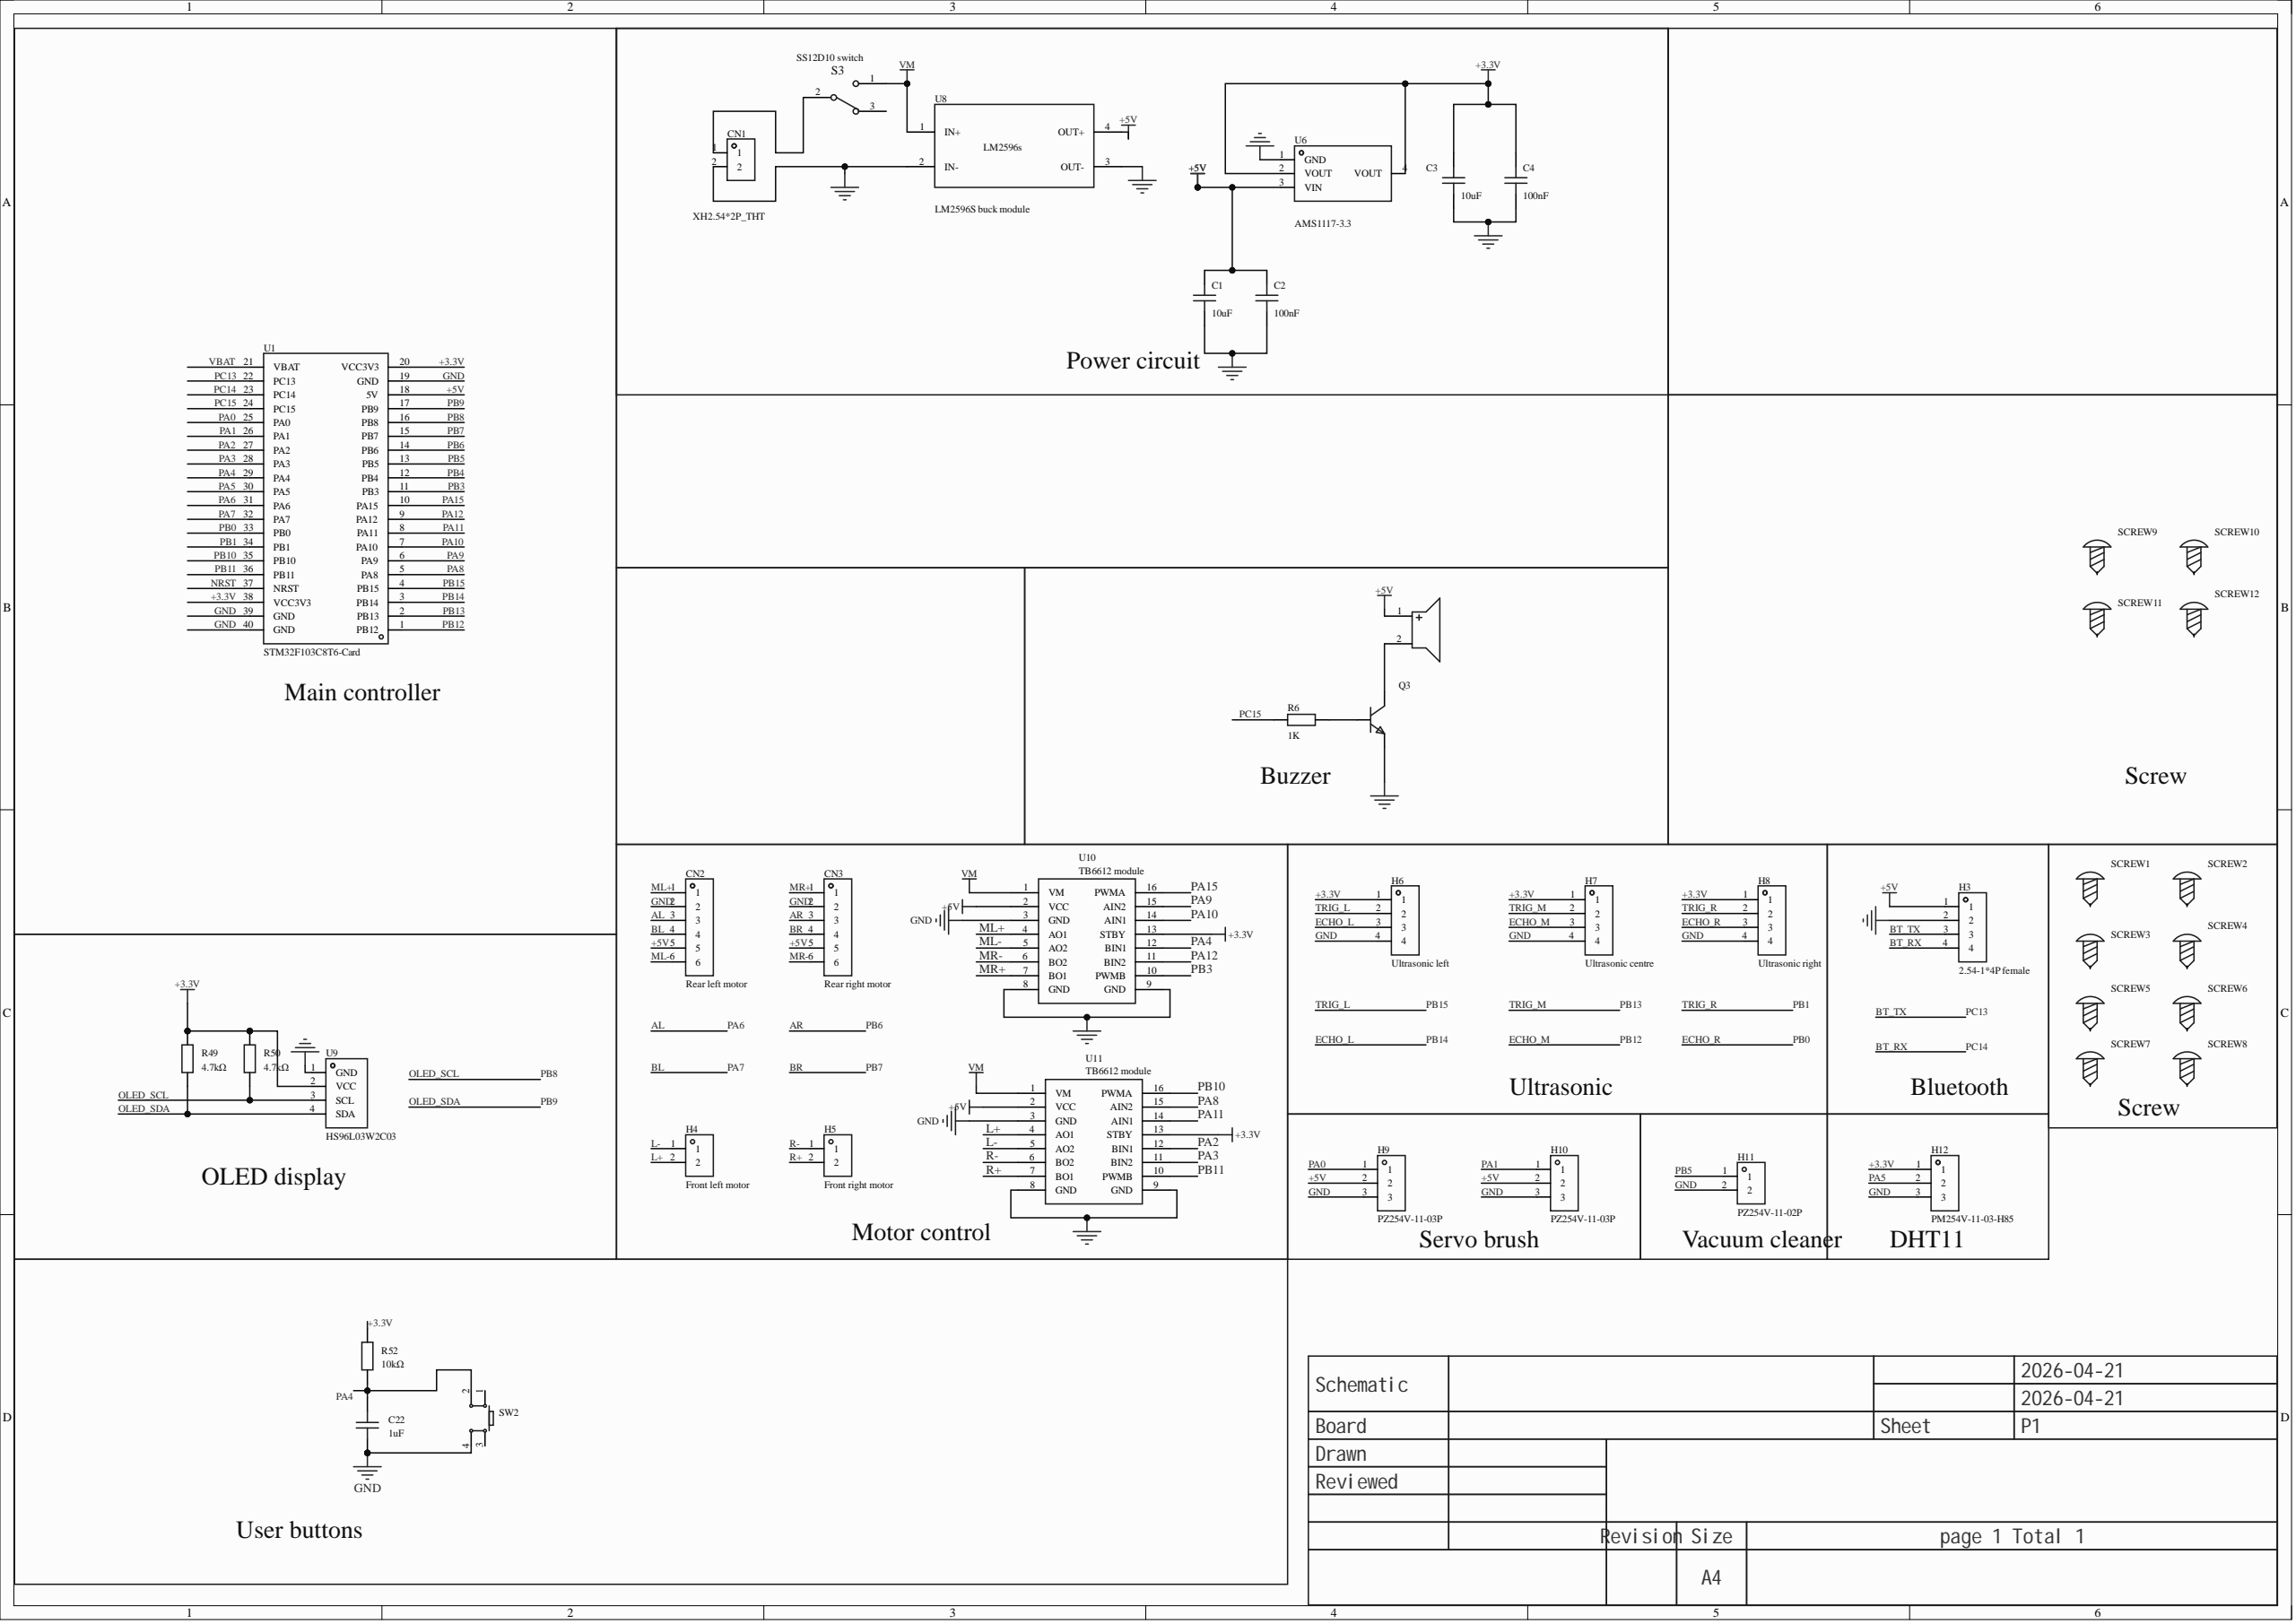Circuit board | Altium Designer | 44 parts | 46 nets
Bill of materials:
Comment,Description,Designator,Footprint,LibRef,Quantity
"2.7kHz","Drive: Passive (external drive); Construction: Electromagnetic; Frequency: 2.7kHz; Sound pressure (SPL): 85dB;","BUZZER1","BUZ-TH_BD9.0-P4.00-D0.6-FD","QMB-09B-03","1"
"10uF","Capacitance: 10uF; Tolerance: ±10%; Rated voltage: 50V; Dielectric (temp. coefficient): X5R;","C1, C3","C0805","GRM21BR61H106KE43L","2"
"100nF","Capacitance: 100nF; Tolerance: ±10%; Rated voltage: 50V; Dielectric (temp. coefficient): X7R;","C2, C4","C0805","CL21B104KBCNNNC","2"
"1uF","Capacitance: 1uF; Tolerance: ±10%; Rated voltage: 50V; Dielectric (temp. coefficient): X5R;","C22","C0603","CL10A105KB8NNNC","1"
"XH2.54*2P_THT","","CN1","CONN-TH_2P-P2.50-XH2.54-2P","XH2.54*2P_直插","1"
"Rear left motor","","CN2","CONN-TH_XH2.54-6P","XH2.54*6P_直插","1"
"Rear right motor","","CN3","CONN-TH_XH2.54-6P","XH2.54*6P_直插","1"
"2.54-1*4P female","","H3","HDR-TH_4P-P2.54-V-F","2.54-1*4P母","1"
"Front left motor","","H4","HDR-TH_2P-P2.54-V-M","PZ254V-11-02P","1"
"Front right motor","","H5","HDR-TH_2P-P2.54-V-M","PZ254V-11-02P","1"
"Ultrasonic left","","H6","HDR-TH_4P-P2.54-V-M","PZ254V-11-04P","1"
"Ultrasonic centre","","H7","HDR-TH_4P-P2.54-V-M","PZ254V-11-04P","1"
"Ultrasonic right","","H8","HDR-TH_4P-P2.54-V-M","PZ254V-11-04P","1"
"PZ254V-11-03P","","H9, H10","HDR-TH_3P-P2.54-V-M","PZ254V-11-03P","2"
"PZ254V-11-02P","","H11","HDR-TH_2P-P2.54-V-M","PZ254V-11-02P","1"
"PM254V-11-03-H85","Socket structure: 1x3P; Pitch: 2.54mm; Row spacing: -; Mounting: THT; Rows: Single row; Total holes: 3P; Body height: -; Contact material: Brass; Contact plating: -;","H12","HDR-TH_3P-P2.54-V-F","PM254V-11-03-H85","1"
"","","Q3","S8050_TO_92","S8050_TO_NPN","1"
"1K","","R6","Res_1/8W","Res_AXIAL-1/8W","1"
"4.7kΩ","Resistor type: Thick-film resistor; Resistance: 4.7kΩ; Tolerance: ±1%; Power: 125mW; Max working voltage: 150V; Temp. coefficient: ±100ppm/?;","R49, R50","R0805","0805W8F4701T5E","2"
"10kΩ","Resistor type: Thick-film resistor; Resistance: 10kΩ; Tolerance: ±1%; Power: 100mW;","R52","R0603","0603WAF1002T5E","1"
"SS12D10 switch","","S3","SS12D10","SS12D10","1"
"","","SCREW1, SCREW2, SCREW3, SCREW4, SCREW9, SCREW10, SCREW11, SCREW12","M3螺丝","M3螺丝","8"
"","","SCREW5, SCREW6, SCREW7, SCREW8","M2螺丝","M2螺丝","4"
"","","SW2","SW-TH_4P-L6.0-W6.0-P4.50-LS6.5","Key_TH_6x6x6","1"
"STM32F103C8T6-Card","","U1","CONN-TH_L53.3-W22.9_STM32F103C8T6-CARD","STM32F103C8T6-Card","1"
"AMS1117-3.3","Output type: Fixed; Output polarity: Positive; Max input voltage: -; Output voltage: 3.3V; Output current: 1A; PSRR: 72dB@(120Hz);","U6","SOT-223-3_L6.5-W3.4-P2.30-LS7.0-BR","AMS1117-3.3_C6186","1"
"LM2596S buck module","","U8","LM2596S","LM2596S","1"
"HS96L03W2C03","Controller: SSD1315; Interface: I2C; Size (inch): 0.96; Pixel resolution: 128x64;","U9","OLED-TH_L27.8-W27.2-P2.54_C9900033791","HS96L03W2C03","1"
"TB6612 module","","U10, U11","TB6612-2X8","TB6612模块","2"
Netlist (Protel format):
[
BUZZER1
BUZ-TH_BD9.0-P4.00-D0.6-FD
2.7kHz



]
[
C1
C0805
10uF



]
[
C2
C0805
100nF



]
[
C3
C0805
10uF



]
[
C4
C0805
100nF



]
[
C22
C0603
1uF



]
[
CN1
CONN-TH_2P-P2.50-XH2.54-2P
XH2.54*2P_THT



]
[
CN2
CONN-TH_XH2.54-6P
Rear left motor



]
[
CN3
CONN-TH_XH2.54-6P
Rear right motor



]
[
H3
HDR-TH_4P-P2.54-V-F
2.54-1*4P female



]
[
H4
HDR-TH_2P-P2.54-V-M
Front left motor



]
[
H5
HDR-TH_2P-P2.54-V-M
Front right motor



]
[
H6
HDR-TH_4P-P2.54-V-M
Ultrasonic left



]
[
H7
HDR-TH_4P-P2.54-V-M
Ultrasonic centre



]
[
H8
HDR-TH_4P-P2.54-V-M
Ultrasonic right



]
[
H9
HDR-TH_3P-P2.54-V-M
PZ254V-11-03P



]
[
H10
HDR-TH_3P-P2.54-V-M
PZ254V-11-03P



]
[
H11
HDR-TH_2P-P2.54-V-M
PZ254V-11-02P



]
[
H12
HDR-TH_3P-P2.54-V-F
PM254V-11-03-H85



]
[
Q3
S8050_TO_92




]
[
R6
Res_1/8W
1K



]
[
R49
R0805
4.7kΩ



]
[
R50
R0805
4.7kΩ



]
[
R52
R0603
10kΩ



]
[
S3
SS12D10
SS12D10 switch



]
[
SCREW1
M3螺丝




]
[
SCREW2
M3螺丝




]
[
SCREW3
M3螺丝




]
[
SCREW4
M3螺丝




]
[
SCREW5
M2螺丝




]
[
SCREW6
M2螺丝




]
[
SCREW7
M2螺丝




]
[
SCREW8
M2螺丝




]
[
SCREW9
M3螺丝




]
[
SCREW10
M3螺丝




]
[
SCREW11
M3螺丝




]
[
SCREW12
M3螺丝




]
[
SW2
SW-TH_4P-L6.0-W6.0-P4.50-LS6.5




]
[
U1
CONN-TH_L53.3-W22.9_STM32F103C8T6-CARD
STM32F103C8T6-Card



]
[
U6
SOT-223-3_L6.5-W3.4-P2.30-LS7.0-BR
AMS1117-3.3



]
[
U8
LM2596S
LM2596S buck module



]
[
U9
OLED-TH_L27.8-W27.2-P2.54_C9900033791
HS96L03W2C03



]
[
U10
TB6612-2X8
TB6612 module



]
[
U11
TB6612-2X8
TB6612 module



]
(
VM
S3-1
U8-1
U10-1
U11-1
)
(
R-
H5-1
U11-6
)
(
R+
H5-2
U11-7
)
(
PC15
R6-1
U1-24
)
(
PB15
H6-2
U1-4
)
(
PB13
H7-2
U1-2
)
(
PB11
U1-36
U11-10
)
(
PB10
U1-35
U11-16
)
(
PB5
H11-1
U1-13
)
(
PB3
U1-11
U10-10
)
(
PB1
H8-2
U1-34
)
(
PA15
U1-10
U10-16
)
(
PA12
U1-9
U10-11
)
(
PA11
U1-8
U11-14
)
(
PA10
U1-7
U10-14
)
(
PA9
U1-6
U10-15
)
(
PA8
U1-5
U11-15
)
(
PA5
H12-2
U1-30
)
(
PA4
C22-2
R52-1
SW2-2
U1-29
U10-12
)
(
PA3
U1-28
U11-11
)
(
PA2
U1-27
U11-12
)
(
PA1
H10-1
U1-26
)
(
PA0
H9-1
U1-25
)
(
OLED_SDA
R49-2
U1-17
U9-4
)
(
OLED_SCL
R50-2
U1-16
U9-3
)
(
NetQ3_2
Q3-2
R6-2
)
(
NetCN1_1
CN1-1
S3-2
)
(
NetBUZZER1_2
BUZZER1-2
Q3-3
)
(
MR-
CN3-6
U10-6
)
(
MR+
CN3-1
U10-7
)
(
ML-
CN2-6
U10-5
)
(
ML+
CN2-1
U10-4
)
(
L-
H4-1
U11-5
)
(
L+
H4-2
U11-4
)
(
GND
C1-1
C2-1
C3-1
C4-1
C22-1
CN1-2
CN2-2
CN3-2
H3-2
H6-4
H7-4
H8-4
H9-3
H10-3
H11-2
H12-3
Q3-1
SW2-4
U1-19
U1-39
U1-40
U6-1
U8-2
U8-3
U9-1
U10-3
U10-8
U10-9
U11-3
U11-8
U11-9
)
(
ECHO_R
H8-3
U1-33
)
(
ECHO_M
H7-3
U1-1
)
(
ECHO_L
H6-3
U1-3
)
(
BT_TX
H3-3
U1-22
)
(
BT_RX
H3-4
U1-23
)
(
BR
CN3-4
U1-15
)
(
BL
CN2-4
U1-32
)
(
AR
CN3-3
U1-14
)
(
AL
CN2-3
U1-31
)
(
+5V
BUZZER1-1
C1-2
C2-2
CN2-5
CN3-5
H3-1
H9-2
H10-2
U1-18
U6-3
U8-4
U10-2
U11-2
)
(
+3.3V
C3-2
C4-2
H6-1
H7-1
H8-1
H12-1
R49-1
R50-1
R52-2
U1-20
U1-38
U6-2
U6-4
U9-2
U10-13
U11-13
)